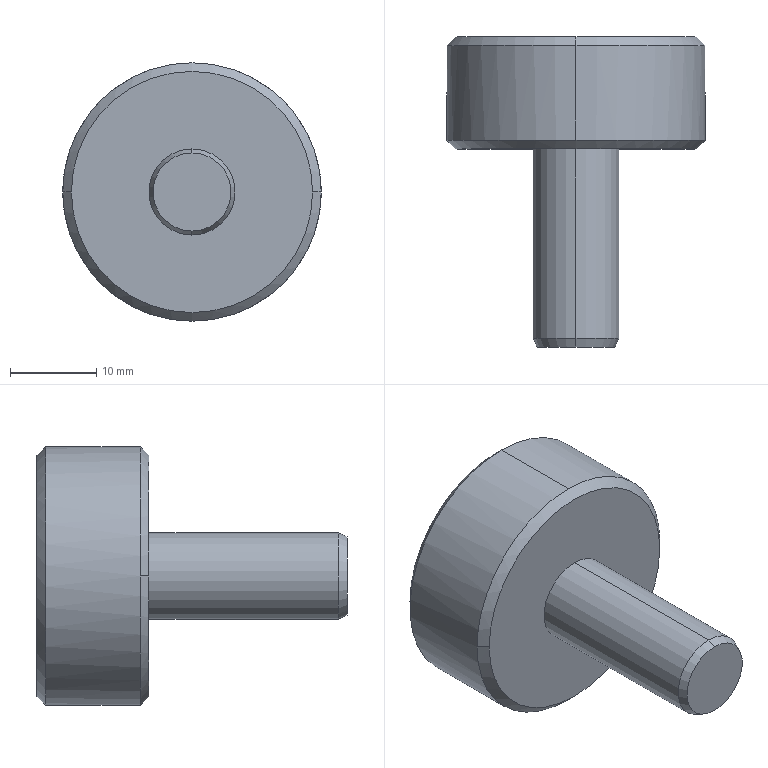Part | SolidWorks | features BaseBody 1 | 1 solid | 16 faces | box 30 x 36 x 30 mm | volume 10405 mm3 | cylinder 6 | cone 6 | plane 4 | commonest cylinder face diameters 10 x2 25 x2 30 x2
STEP:
#1=CARTESIAN_POINT('',(-418.,-55.,202.121));
#2=VERTEX_POINT('',#1);
#3=CARTESIAN_POINT('',(-418.,-55.,192.121));
#4=VERTEX_POINT('',#3);
#5=CARTESIAN_POINT('',(-418.,-55.,197.121));
#6=DIRECTION('',(0.,1.,0.));
#7=DIRECTION('',(0.,0.,-1.));
#8=AXIS2_PLACEMENT_3D('',#5,#6,#7);
#9=CIRCLE('',#8,5.);
#10=EDGE_CURVE('',#2,#4,#9,.T.);
#11=ORIENTED_EDGE('',*,*,#10,.F.);
#12=CARTESIAN_POINT('',(-418.,-77.,202.121));
#13=VERTEX_POINT('',#12);
#14=CARTESIAN_POINT('',(-418.,-78.,202.121));
#15=DIRECTION('',(0.,-1.,0.));
#16=VECTOR('',#15,1000.);
#17=LINE('',#14,#16);
#18=EDGE_CURVE('',#2,#13,#17,.T.);
#19=ORIENTED_EDGE('',*,*,#18,.T.);
#20=CARTESIAN_POINT('',(-418.,-77.,192.121));
#21=VERTEX_POINT('',#20);
#22=CARTESIAN_POINT('',(-418.,-77.,197.121));
#23=DIRECTION('',(0.,1.,0.));
#24=DIRECTION('',(0.,0.,-1.));
#25=AXIS2_PLACEMENT_3D('',#22,#23,#24);
#26=CIRCLE('',#25,5.);
#27=EDGE_CURVE('',#13,#21,#26,.T.);
#28=ORIENTED_EDGE('',*,*,#27,.T.);
#29=CARTESIAN_POINT('',(-418.,-78.,192.121));
#30=DIRECTION('',(0.,-1.,0.));
#31=VECTOR('',#30,1000.);
#32=LINE('',#29,#31);
#33=EDGE_CURVE('',#4,#21,#32,.T.);
#34=ORIENTED_EDGE('',*,*,#33,.F.);
#35=EDGE_LOOP('',(#11,#19,#28,#34));
#36=FACE_OUTER_BOUND('',#35,.T.);
#37=CARTESIAN_POINT('',(-418.,-78.,197.121));
#38=DIRECTION('',(0.,-1.,0.));
#39=DIRECTION('',(0.,0.,-1.));
#40=AXIS2_PLACEMENT_3D('',#37,#38,#39);
#41=CYLINDRICAL_SURFACE('',#40,5.);
#42=ADVANCED_FACE('',(#36),#41,.T.);
#43=CARTESIAN_POINT('',(-404.,-55.,197.121));
#44=VERTEX_POINT('',#43);
#45=CARTESIAN_POINT('',(-432.,-55.,197.121));
#46=VERTEX_POINT('',#45);
#47=CARTESIAN_POINT('',(-418.,-55.,197.121));
#48=DIRECTION('',(0.,-1.,0.));
#49=DIRECTION('',(-1.,0.,0.));
#50=AXIS2_PLACEMENT_3D('',#47,#48,#49);
#51=CIRCLE('',#50,14.);
#52=EDGE_CURVE('',#44,#46,#51,.T.);
#53=ORIENTED_EDGE('',*,*,#52,.F.);
#54=CARTESIAN_POINT('',(-403.,-54.,197.121));
#55=VERTEX_POINT('',#54);
#56=CARTESIAN_POINT('',(-403.,-54.,197.121));
#57=DIRECTION('',(0.7071,0.7071,0.));
#58=VECTOR('',#57,1000.);
#59=LINE('',#56,#58);
#60=EDGE_CURVE('',#44,#55,#59,.T.);
#61=ORIENTED_EDGE('',*,*,#60,.T.);
#62=CARTESIAN_POINT('',(-418.,-54.,212.121));
#63=VERTEX_POINT('',#62);
#64=CARTESIAN_POINT('',(-418.,-54.,197.121));
#65=DIRECTION('',(0.,-1.,0.));
#66=DIRECTION('',(0.,0.,-1.));
#67=AXIS2_PLACEMENT_3D('',#64,#65,#66);
#68=CIRCLE('',#67,15.);
#69=EDGE_CURVE('',#55,#63,#68,.T.);
#70=ORIENTED_EDGE('',*,*,#69,.T.);
#71=CARTESIAN_POINT('',(-433.,-54.,197.121));
#72=VERTEX_POINT('',#71);
#73=CARTESIAN_POINT('',(-418.,-54.,197.121));
#74=DIRECTION('',(0.,-1.,0.));
#75=DIRECTION('',(0.,0.,-1.));
#76=AXIS2_PLACEMENT_3D('',#73,#74,#75);
#77=CIRCLE('',#76,15.);
#78=EDGE_CURVE('',#63,#72,#77,.T.);
#79=ORIENTED_EDGE('',*,*,#78,.T.);
#80=CARTESIAN_POINT('',(-433.,-54.,197.121));
#81=DIRECTION('',(-0.7071,0.7071,0.));
#82=VECTOR('',#81,1000.);
#83=LINE('',#80,#82);
#84=EDGE_CURVE('',#46,#72,#83,.T.);
#85=ORIENTED_EDGE('',*,*,#84,.F.);
#86=EDGE_LOOP('',(#53,#61,#70,#79,#85));
#87=FACE_OUTER_BOUND('',#86,.T.);
#88=CARTESIAN_POINT('',(-418.,-54.,197.121));
#89=DIRECTION('',(0.,1.,0.));
#90=DIRECTION('',(-1.,0.,0.));
#91=AXIS2_PLACEMENT_3D('',#88,#89,#90);
#92=CONICAL_SURFACE('',#91,15.,0.7854);
#93=ADVANCED_FACE('',(#87),#92,.T.);
#94=CARTESIAN_POINT('',(-418.,-78.,201.655));
#95=VERTEX_POINT('',#94);
#96=CARTESIAN_POINT('',(-418.,-78.,192.587));
#97=VERTEX_POINT('',#96);
#98=CARTESIAN_POINT('',(-418.,-78.,197.121));
#99=DIRECTION('',(0.,1.,0.));
#100=DIRECTION('',(0.,0.,1.));
#101=AXIS2_PLACEMENT_3D('',#98,#99,#100);
#102=CIRCLE('',#101,4.534);
#103=EDGE_CURVE('',#95,#97,#102,.T.);
#104=ORIENTED_EDGE('',*,*,#103,.T.);
#105=CARTESIAN_POINT('',(-418.,-77.,192.121));
#106=DIRECTION('',(0.,0.9063,-0.4226));
#107=VECTOR('',#106,1000.);
#108=LINE('',#105,#107);
#109=EDGE_CURVE('',#97,#21,#108,.T.);
#110=ORIENTED_EDGE('',*,*,#109,.T.);
#111=ORIENTED_EDGE('',*,*,#27,.F.);
#112=CARTESIAN_POINT('',(-418.,-77.,202.121));
#113=DIRECTION('',(0.,0.9063,0.4226));
#114=VECTOR('',#113,1000.);
#115=LINE('',#112,#114);
#116=EDGE_CURVE('',#95,#13,#115,.T.);
#117=ORIENTED_EDGE('',*,*,#116,.F.);
#118=EDGE_LOOP('',(#104,#110,#111,#117));
#119=FACE_OUTER_BOUND('',#118,.T.);
#120=CARTESIAN_POINT('',(-418.,-77.,197.121));
#121=DIRECTION('',(0.,1.,0.));
#122=DIRECTION('',(0.,0.,1.));
#123=AXIS2_PLACEMENT_3D('',#120,#121,#122);
#124=CONICAL_SURFACE('',#123,5.,0.4363);
#125=ADVANCED_FACE('',(#119),#124,.T.);
#126=CARTESIAN_POINT('',(-418.,-43.,182.121));
#127=VERTEX_POINT('',#126);
#128=CARTESIAN_POINT('',(-418.,-43.,212.121));
#129=VERTEX_POINT('',#128);
#130=CARTESIAN_POINT('',(-418.,-43.,197.121));
#131=DIRECTION('',(0.,-1.,0.));
#132=DIRECTION('',(0.,0.,-1.));
#133=AXIS2_PLACEMENT_3D('',#130,#131,#132);
#134=CIRCLE('',#133,15.);
#135=EDGE_CURVE('',#127,#129,#134,.T.);
#136=ORIENTED_EDGE('',*,*,#135,.T.);
#137=CARTESIAN_POINT('',(-418.,-78.,212.121));
#138=DIRECTION('',(0.,-1.,0.));
#139=VECTOR('',#138,1000.);
#140=LINE('',#137,#139);
#141=EDGE_CURVE('',#129,#63,#140,.T.);
#142=ORIENTED_EDGE('',*,*,#141,.T.);
#143=ORIENTED_EDGE('',*,*,#69,.F.);
#144=CARTESIAN_POINT('',(-418.,-54.,182.121));
#145=VERTEX_POINT('',#144);
#146=CARTESIAN_POINT('',(-418.,-54.,197.121));
#147=DIRECTION('',(0.,-1.,0.));
#148=DIRECTION('',(0.,0.,-1.));
#149=AXIS2_PLACEMENT_3D('',#146,#147,#148);
#150=CIRCLE('',#149,15.);
#151=EDGE_CURVE('',#145,#55,#150,.T.);
#152=ORIENTED_EDGE('',*,*,#151,.F.);
#153=CARTESIAN_POINT('',(-418.,-78.,182.121));
#154=DIRECTION('',(0.,-1.,0.));
#155=VECTOR('',#154,1000.);
#156=LINE('',#153,#155);
#157=EDGE_CURVE('',#127,#145,#156,.T.);
#158=ORIENTED_EDGE('',*,*,#157,.F.);
#159=EDGE_LOOP('',(#136,#142,#143,#152,#158));
#160=FACE_OUTER_BOUND('',#159,.T.);
#161=CARTESIAN_POINT('',(-418.,-78.,197.121));
#162=DIRECTION('',(0.,-1.,0.));
#163=DIRECTION('',(0.,0.,-1.));
#164=AXIS2_PLACEMENT_3D('',#161,#162,#163);
#165=CYLINDRICAL_SURFACE('',#164,15.);
#166=ADVANCED_FACE('',(#160),#165,.T.);
#167=CARTESIAN_POINT('',(-418.,-42.,183.121));
#168=VERTEX_POINT('',#167);
#169=CARTESIAN_POINT('',(-418.,-42.,211.121));
#170=VERTEX_POINT('',#169);
#171=CARTESIAN_POINT('',(-418.,-42.,197.121));
#172=DIRECTION('',(0.,-1.,0.));
#173=DIRECTION('',(0.,0.,-1.));
#174=AXIS2_PLACEMENT_3D('',#171,#172,#173);
#175=CIRCLE('',#174,14.);
#176=EDGE_CURVE('',#168,#170,#175,.T.);
#177=ORIENTED_EDGE('',*,*,#176,.T.);
#178=CARTESIAN_POINT('',(-418.,-43.,212.121));
#179=DIRECTION('',(0.,-0.7071,0.7071));
#180=VECTOR('',#179,1000.);
#181=LINE('',#178,#180);
#182=EDGE_CURVE('',#170,#129,#181,.T.);
#183=ORIENTED_EDGE('',*,*,#182,.T.);
#184=ORIENTED_EDGE('',*,*,#135,.F.);
#185=CARTESIAN_POINT('',(-418.,-43.,182.121));
#186=DIRECTION('',(0.,-0.7071,-0.7071));
#187=VECTOR('',#186,1000.);
#188=LINE('',#185,#187);
#189=EDGE_CURVE('',#168,#127,#188,.T.);
#190=ORIENTED_EDGE('',*,*,#189,.F.);
#191=EDGE_LOOP('',(#177,#183,#184,#190));
#192=FACE_OUTER_BOUND('',#191,.T.);
#193=CARTESIAN_POINT('',(-418.,-43.,197.121));
#194=DIRECTION('',(0.,-1.,0.));
#195=DIRECTION('',(0.,0.,-1.));
#196=AXIS2_PLACEMENT_3D('',#193,#194,#195);
#197=CONICAL_SURFACE('',#196,15.,0.7854);
#198=ADVANCED_FACE('',(#192),#197,.T.);
#199=CARTESIAN_POINT('',(-418.,-43.,184.621));
#200=VERTEX_POINT('',#199);
#201=CARTESIAN_POINT('',(-418.,-43.,209.621));
#202=VERTEX_POINT('',#201);
#203=CARTESIAN_POINT('',(-418.,-43.,197.121));
#204=DIRECTION('',(0.,1.,0.));
#205=DIRECTION('',(0.,0.,1.));
#206=AXIS2_PLACEMENT_3D('',#203,#204,#205);
#207=CIRCLE('',#206,12.5);
#208=EDGE_CURVE('',#200,#202,#207,.T.);
#209=ORIENTED_EDGE('',*,*,#208,.F.);
#210=CARTESIAN_POINT('',(-418.,-42.,184.621));
#211=VERTEX_POINT('',#210);
#212=CARTESIAN_POINT('',(-418.,-43.,184.621));
#213=DIRECTION('',(0.,1.,0.));
#214=VECTOR('',#213,1000.);
#215=LINE('',#212,#214);
#216=EDGE_CURVE('',#200,#211,#215,.T.);
#217=ORIENTED_EDGE('',*,*,#216,.T.);
#218=CARTESIAN_POINT('',(-418.,-42.,209.621));
#219=VERTEX_POINT('',#218);
#220=CARTESIAN_POINT('',(-418.,-42.,197.121));
#221=DIRECTION('',(0.,-1.,0.));
#222=DIRECTION('',(0.,0.,1.));
#223=AXIS2_PLACEMENT_3D('',#220,#221,#222);
#224=CIRCLE('',#223,12.5);
#225=EDGE_CURVE('',#219,#211,#224,.T.);
#226=ORIENTED_EDGE('',*,*,#225,.F.);
#227=CARTESIAN_POINT('',(-418.,-43.,209.621));
#228=DIRECTION('',(0.,1.,0.));
#229=VECTOR('',#228,1000.);
#230=LINE('',#227,#229);
#231=EDGE_CURVE('',#202,#219,#230,.T.);
#232=ORIENTED_EDGE('',*,*,#231,.F.);
#233=EDGE_LOOP('',(#209,#217,#226,#232));
#234=FACE_OUTER_BOUND('',#233,.T.);
#235=CARTESIAN_POINT('',(-418.,-43.,197.121));
#236=DIRECTION('',(0.,1.,0.));
#237=DIRECTION('',(0.,0.,1.));
#238=AXIS2_PLACEMENT_3D('',#235,#236,#237);
#239=CYLINDRICAL_SURFACE('',#238,12.5);
#240=ADVANCED_FACE('',(#234),#239,.F.);
#241=CARTESIAN_POINT('',(-418.,-55.,197.121));
#242=DIRECTION('',(0.,1.,0.));
#243=DIRECTION('',(0.,0.,-1.));
#244=AXIS2_PLACEMENT_3D('',#241,#242,#243);
#245=CIRCLE('',#244,5.);
#246=EDGE_CURVE('',#4,#2,#245,.T.);
#247=ORIENTED_EDGE('',*,*,#246,.T.);
#248=ORIENTED_EDGE('',*,*,#10,.T.);
#249=EDGE_LOOP('',(#247,#248));
#250=FACE_BOUND('',#249,.T.);
#251=CARTESIAN_POINT('',(-418.,-55.,197.121));
#252=DIRECTION('',(0.,-1.,0.));
#253=DIRECTION('',(-1.,0.,0.));
#254=AXIS2_PLACEMENT_3D('',#251,#252,#253);
#255=CIRCLE('',#254,14.);
#256=EDGE_CURVE('',#46,#44,#255,.T.);
#257=ORIENTED_EDGE('',*,*,#256,.T.);
#258=ORIENTED_EDGE('',*,*,#52,.T.);
#259=EDGE_LOOP('',(#257,#258));
#260=FACE_OUTER_BOUND('',#259,.T.);
#261=CARTESIAN_POINT('',(-418.,-55.,212.121));
#262=DIRECTION('',(0.,-1.,0.));
#263=DIRECTION('',(0.,0.,-1.));
#264=AXIS2_PLACEMENT_3D('',#261,#262,#263);
#265=PLANE('',#264);
#266=ADVANCED_FACE('',(#250,#260),#265,.T.);
#267=ORIENTED_EDGE('',*,*,#18,.F.);
#268=ORIENTED_EDGE('',*,*,#246,.F.);
#269=ORIENTED_EDGE('',*,*,#33,.T.);
#270=CARTESIAN_POINT('',(-418.,-77.,197.121));
#271=DIRECTION('',(0.,1.,0.));
#272=DIRECTION('',(0.,0.,-1.));
#273=AXIS2_PLACEMENT_3D('',#270,#271,#272);
#274=CIRCLE('',#273,5.);
#275=EDGE_CURVE('',#21,#13,#274,.T.);
#276=ORIENTED_EDGE('',*,*,#275,.T.);
#277=EDGE_LOOP('',(#267,#268,#269,#276));
#278=FACE_OUTER_BOUND('',#277,.T.);
#279=CARTESIAN_POINT('',(-418.,-78.,197.121));
#280=DIRECTION('',(0.,-1.,0.));
#281=DIRECTION('',(0.,0.,-1.));
#282=AXIS2_PLACEMENT_3D('',#279,#280,#281);
#283=CYLINDRICAL_SURFACE('',#282,5.);
#284=ADVANCED_FACE('',(#278),#283,.T.);
#285=ORIENTED_EDGE('',*,*,#60,.F.);
#286=ORIENTED_EDGE('',*,*,#256,.F.);
#287=ORIENTED_EDGE('',*,*,#84,.T.);
#288=CARTESIAN_POINT('',(-418.,-54.,197.121));
#289=DIRECTION('',(0.,-1.,0.));
#290=DIRECTION('',(0.,0.,-1.));
#291=AXIS2_PLACEMENT_3D('',#288,#289,#290);
#292=CIRCLE('',#291,15.);
#293=EDGE_CURVE('',#72,#145,#292,.T.);
#294=ORIENTED_EDGE('',*,*,#293,.T.);
#295=ORIENTED_EDGE('',*,*,#151,.T.);
#296=EDGE_LOOP('',(#285,#286,#287,#294,#295));
#297=FACE_OUTER_BOUND('',#296,.T.);
#298=CARTESIAN_POINT('',(-418.,-54.,197.121));
#299=DIRECTION('',(0.,1.,0.));
#300=DIRECTION('',(-1.,0.,0.));
#301=AXIS2_PLACEMENT_3D('',#298,#299,#300);
#302=CONICAL_SURFACE('',#301,15.,0.7854);
#303=ADVANCED_FACE('',(#297),#302,.T.);
#304=ORIENTED_EDGE('',*,*,#109,.F.);
#305=CARTESIAN_POINT('',(-418.,-78.,197.121));
#306=DIRECTION('',(0.,1.,0.));
#307=DIRECTION('',(0.,0.,1.));
#308=AXIS2_PLACEMENT_3D('',#305,#306,#307);
#309=CIRCLE('',#308,4.534);
#310=EDGE_CURVE('',#97,#95,#309,.T.);
#311=ORIENTED_EDGE('',*,*,#310,.T.);
#312=ORIENTED_EDGE('',*,*,#116,.T.);
#313=ORIENTED_EDGE('',*,*,#275,.F.);
#314=EDGE_LOOP('',(#304,#311,#312,#313));
#315=FACE_OUTER_BOUND('',#314,.T.);
#316=CARTESIAN_POINT('',(-418.,-77.,197.121));
#317=DIRECTION('',(0.,1.,0.));
#318=DIRECTION('',(0.,0.,1.));
#319=AXIS2_PLACEMENT_3D('',#316,#317,#318);
#320=CONICAL_SURFACE('',#319,5.,0.4363);
#321=ADVANCED_FACE('',(#315),#320,.T.);
#322=ORIENTED_EDGE('',*,*,#141,.F.);
#323=CARTESIAN_POINT('',(-418.,-43.,197.121));
#324=DIRECTION('',(0.,-1.,0.));
#325=DIRECTION('',(0.,0.,-1.));
#326=AXIS2_PLACEMENT_3D('',#323,#324,#325);
#327=CIRCLE('',#326,15.);
#328=EDGE_CURVE('',#129,#127,#327,.T.);
#329=ORIENTED_EDGE('',*,*,#328,.T.);
#330=ORIENTED_EDGE('',*,*,#157,.T.);
#331=ORIENTED_EDGE('',*,*,#293,.F.);
#332=ORIENTED_EDGE('',*,*,#78,.F.);
#333=EDGE_LOOP('',(#322,#329,#330,#331,#332));
#334=FACE_OUTER_BOUND('',#333,.T.);
#335=CARTESIAN_POINT('',(-418.,-78.,197.121));
#336=DIRECTION('',(0.,-1.,0.));
#337=DIRECTION('',(0.,0.,-1.));
#338=AXIS2_PLACEMENT_3D('',#335,#336,#337);
#339=CYLINDRICAL_SURFACE('',#338,15.);
#340=ADVANCED_FACE('',(#334),#339,.T.);
#341=ORIENTED_EDGE('',*,*,#103,.F.);
#342=ORIENTED_EDGE('',*,*,#310,.F.);
#343=EDGE_LOOP('',(#341,#342));
#344=FACE_OUTER_BOUND('',#343,.T.);
#345=CARTESIAN_POINT('',(-418.,-78.,202.121));
#346=DIRECTION('',(0.,-1.,0.));
#347=DIRECTION('',(0.,0.,-1.));
#348=AXIS2_PLACEMENT_3D('',#345,#346,#347);
#349=PLANE('',#348);
#350=ADVANCED_FACE('',(#344),#349,.T.);
#351=ORIENTED_EDGE('',*,*,#182,.F.);
#352=CARTESIAN_POINT('',(-418.,-42.,197.121));
#353=DIRECTION('',(0.,-1.,0.));
#354=DIRECTION('',(0.,0.,-1.));
#355=AXIS2_PLACEMENT_3D('',#352,#353,#354);
#356=CIRCLE('',#355,14.);
#357=EDGE_CURVE('',#170,#168,#356,.T.);
#358=ORIENTED_EDGE('',*,*,#357,.T.);
#359=ORIENTED_EDGE('',*,*,#189,.T.);
#360=ORIENTED_EDGE('',*,*,#328,.F.);
#361=EDGE_LOOP('',(#351,#358,#359,#360));
#362=FACE_OUTER_BOUND('',#361,.T.);
#363=CARTESIAN_POINT('',(-418.,-43.,197.121));
#364=DIRECTION('',(0.,-1.,0.));
#365=DIRECTION('',(0.,0.,-1.));
#366=AXIS2_PLACEMENT_3D('',#363,#364,#365);
#367=CONICAL_SURFACE('',#366,15.,0.7854);
#368=ADVANCED_FACE('',(#362),#367,.T.);
#369=ORIENTED_EDGE('',*,*,#176,.F.);
#370=ORIENTED_EDGE('',*,*,#357,.F.);
#371=EDGE_LOOP('',(#369,#370));
#372=FACE_OUTER_BOUND('',#371,.T.);
#373=ORIENTED_EDGE('',*,*,#225,.T.);
#374=CARTESIAN_POINT('',(-418.,-42.,197.121));
#375=DIRECTION('',(0.,-1.,0.));
#376=DIRECTION('',(0.,0.,1.));
#377=AXIS2_PLACEMENT_3D('',#374,#375,#376);
#378=CIRCLE('',#377,12.5);
#379=EDGE_CURVE('',#211,#219,#378,.T.);
#380=ORIENTED_EDGE('',*,*,#379,.T.);
#381=EDGE_LOOP('',(#373,#380));
#382=FACE_BOUND('',#381,.T.);
#383=CARTESIAN_POINT('',(-418.,-42.,197.121));
#384=DIRECTION('',(0.,1.,0.));
#385=DIRECTION('',(0.,0.,1.));
#386=AXIS2_PLACEMENT_3D('',#383,#384,#385);
#387=PLANE('',#386);
#388=ADVANCED_FACE('',(#372,#382),#387,.T.);
#389=ORIENTED_EDGE('',*,*,#216,.F.);
#390=CARTESIAN_POINT('',(-418.,-43.,197.121));
#391=DIRECTION('',(0.,1.,0.));
#392=DIRECTION('',(0.,0.,1.));
#393=AXIS2_PLACEMENT_3D('',#390,#391,#392);
#394=CIRCLE('',#393,12.5);
#395=EDGE_CURVE('',#202,#200,#394,.T.);
#396=ORIENTED_EDGE('',*,*,#395,.F.);
#397=ORIENTED_EDGE('',*,*,#231,.T.);
#398=ORIENTED_EDGE('',*,*,#379,.F.);
#399=EDGE_LOOP('',(#389,#396,#397,#398));
#400=FACE_OUTER_BOUND('',#399,.T.);
#401=CARTESIAN_POINT('',(-418.,-43.,197.121));
#402=DIRECTION('',(0.,1.,0.));
#403=DIRECTION('',(0.,0.,1.));
#404=AXIS2_PLACEMENT_3D('',#401,#402,#403);
#405=CYLINDRICAL_SURFACE('',#404,12.5);
#406=ADVANCED_FACE('',(#400),#405,.F.);
#407=ORIENTED_EDGE('',*,*,#395,.T.);
#408=ORIENTED_EDGE('',*,*,#208,.T.);
#409=EDGE_LOOP('',(#407,#408));
#410=FACE_OUTER_BOUND('',#409,.T.);
#411=CARTESIAN_POINT('',(-418.,-43.,197.121));
#412=DIRECTION('',(0.,1.,0.));
#413=DIRECTION('',(0.,0.,1.));
#414=AXIS2_PLACEMENT_3D('',#411,#412,#413);
#415=PLANE('',#414);
#416=ADVANCED_FACE('',(#410),#415,.T.);
#417=CLOSED_SHELL('',(#42,#93,#125,#166,#198,#240,#266,#284,#303,#321,#340,#350,#368,#388,#406,#416));
#418=MANIFOLD_SOLID_BREP('',#417);
#419=CARTESIAN_POINT('',(0.,0.,0.));
#420=DIRECTION('',(0.,0.,1.));
#421=DIRECTION('',(1.,0.,0.));
#422=AXIS2_PLACEMENT_3D('',#419,#420,#421);
#423=(LENGTH_UNIT()NAMED_UNIT(*)SI_UNIT(.MILLI.,.METRE.));
#424=UNCERTAINTY_MEASURE_WITH_UNIT(LENGTH_MEASURE(0.00001),#423,'','');
#425=(NAMED_UNIT(*)PLANE_ANGLE_UNIT()SI_UNIT($,.RADIAN.));
#426=(NAMED_UNIT(*)SI_UNIT($,.STERADIAN.)SOLID_ANGLE_UNIT());
#427=(GEOMETRIC_REPRESENTATION_CONTEXT(3)GLOBAL_UNCERTAINTY_ASSIGNED_CONTEXT((#424))GLOBAL_UNIT_ASSIGNED_CONTEXT((#423,#425,#426))REPRESENTATION_CONTEXT('',''));
#428=ADVANCED_BREP_SHAPE_REPRESENTATION('',(#418,#422),#427);